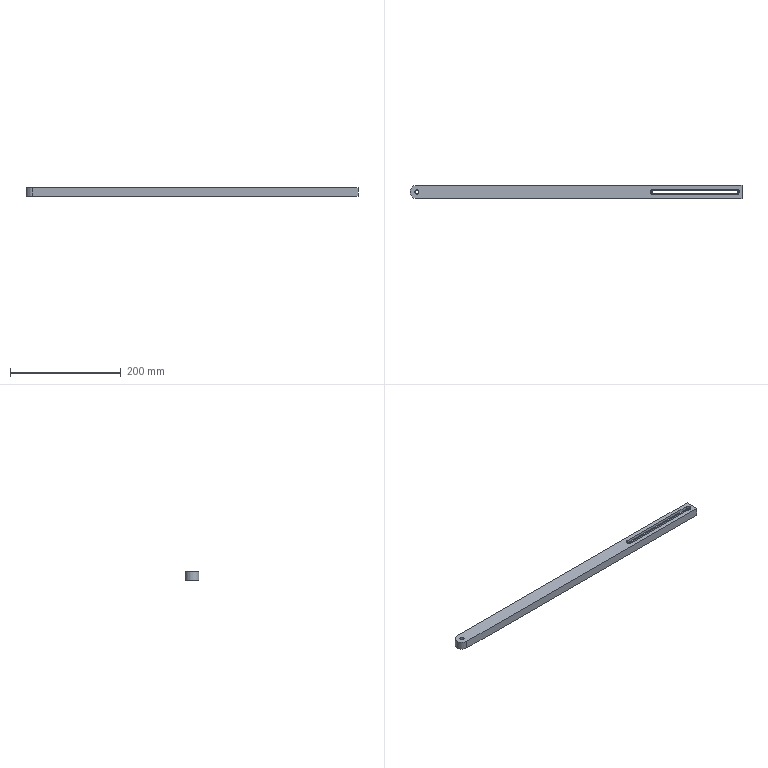Part | STEP file | Feed swing arm | 1 solid | 26 faces | box 600 x 25 x 15 mm | volume 204711 mm3 | cylinder 11 | plane 11 | cone 4 | commonest cylinder face diameters 6 x3 10.2 x3 6.5 x2 15 x2 25 x1